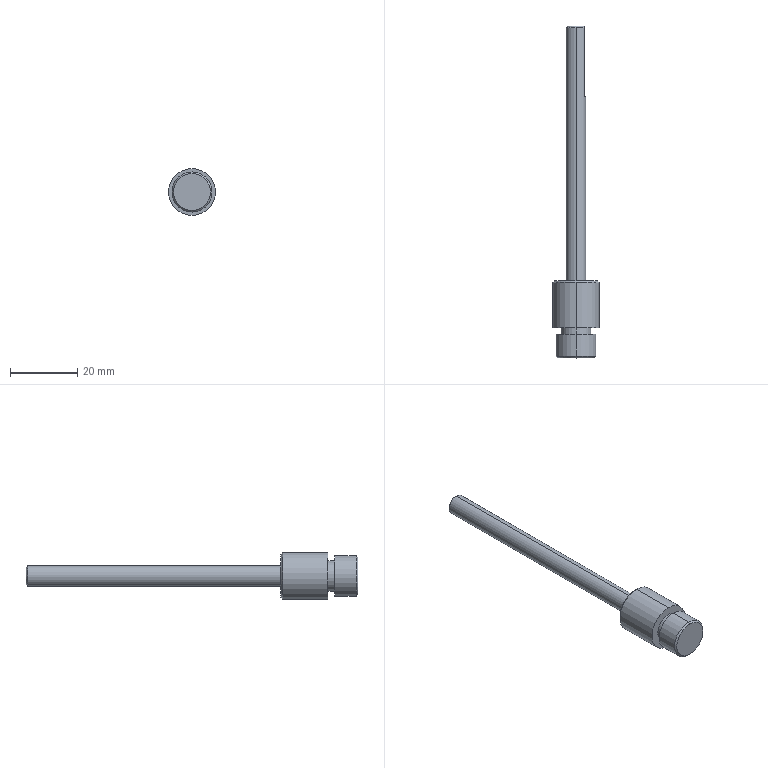Part | STEP file | 1 solid | 22 faces | box 14 x 99 x 14 mm | volume 5187 mm3 | cylinder 8 | cone 7 | plane 7 | commonest cylinder face diameters 6 x2 9 x2 12 x2 14 x2
STEP:
#1=CARTESIAN_POINT('',(0.,0.,0.));
#2=DIRECTION('',(0.,0.,1.));
#3=DIRECTION('',(1.,0.,0.));
#4=AXIS2_PLACEMENT_3D('',#1,#2,#3);
#5=CARTESIAN_POINT('',(0.,-9.,-5.5));
#6=VERTEX_POINT('',#5);
#7=CARTESIAN_POINT('',(0.,-9.,5.5));
#8=VERTEX_POINT('',#7);
#9=CARTESIAN_POINT('',(0.,-9.,0.));
#10=DIRECTION('',(0.,-1.,0.));
#11=DIRECTION('',(0.,0.,-1.));
#12=AXIS2_PLACEMENT_3D('',#9,#10,#11);
#13=CIRCLE('',#12,5.5);
#14=CARTESIAN_POINT('',(0.,-9.,0.));
#15=DIRECTION('',(0.,1.,0.));
#16=DIRECTION('',(0.,0.,1.));
#17=AXIS2_PLACEMENT_3D('',#14,#15,#16);
#18=CONICAL_SURFACE('',#17,5.5,0.7854);
#19=CARTESIAN_POINT('',(3.142,0.));
#20=DIRECTION('',(-1.,0.));
#21=VECTOR('',#20,1.);
#22=LINE('',#19,#21);
#23=(GEOMETRIC_REPRESENTATION_CONTEXT(2)PARAMETRIC_REPRESENTATION_CONTEXT()REPRESENTATION_CONTEXT('',''));
#24=DEFINITIONAL_REPRESENTATION('',(#22),#23);
#25=PCURVE('',#18,#24);
#26=CARTESIAN_POINT('',(0.,-9.,0.));
#27=DIRECTION('',(0.,-1.,0.));
#28=DIRECTION('',(0.,0.,-1.));
#29=AXIS2_PLACEMENT_3D('',#26,#27,#28);
#30=PLANE('',#29);
#31=CARTESIAN_POINT('',(0.,0.));
#32=DIRECTION('',(1.,0.));
#33=AXIS2_PLACEMENT_2D('',#31,#32);
#34=CIRCLE('',#33,5.5);
#35=(GEOMETRIC_REPRESENTATION_CONTEXT(2)PARAMETRIC_REPRESENTATION_CONTEXT()REPRESENTATION_CONTEXT('',''));
#36=DEFINITIONAL_REPRESENTATION('',(#34),#35);
#37=PCURVE('',#30,#36);
#38=SURFACE_CURVE('',#13,(#25,#37),.PCURVE_S1.);
#39=EDGE_CURVE('',#6,#8,#38,.T.);
#40=ORIENTED_EDGE('',*,*,#39,.F.);
#41=CARTESIAN_POINT('',(0.,-8.5,-6.));
#42=VERTEX_POINT('',#41);
#43=CARTESIAN_POINT('',(0.,-9.,-5.5));
#44=DIRECTION('',(0.,0.7071,-0.7071));
#45=VECTOR('',#44,1.);
#46=LINE('',#43,#45);
#47=CARTESIAN_POINT('',(3.142,0.));
#48=DIRECTION('',(0.,1.));
#49=VECTOR('',#48,1.);
#50=LINE('',#47,#49);
#51=(GEOMETRIC_REPRESENTATION_CONTEXT(2)PARAMETRIC_REPRESENTATION_CONTEXT()REPRESENTATION_CONTEXT('',''));
#52=DEFINITIONAL_REPRESENTATION('',(#50),#51);
#53=PCURVE('',#18,#52);
#54=CARTESIAN_POINT('',(0.,-9.,0.));
#55=DIRECTION('',(0.,1.,0.));
#56=DIRECTION('',(0.,0.,1.));
#57=AXIS2_PLACEMENT_3D('',#54,#55,#56);
#58=CONICAL_SURFACE('',#57,5.5,0.7854);
#59=CARTESIAN_POINT('',(3.142,0.));
#60=DIRECTION('',(0.,1.));
#61=VECTOR('',#60,1.);
#62=LINE('',#59,#61);
#63=(GEOMETRIC_REPRESENTATION_CONTEXT(2)PARAMETRIC_REPRESENTATION_CONTEXT()REPRESENTATION_CONTEXT('',''));
#64=DEFINITIONAL_REPRESENTATION('',(#62),#63);
#65=PCURVE('',#58,#64);
#66=SURFACE_CURVE('',#46,(#53,#65),.PCURVE_S1.);
#67=EDGE_CURVE('',#6,#42,#66,.T.);
#68=ORIENTED_EDGE('',*,*,#67,.T.);
#69=CARTESIAN_POINT('',(0.,-8.5,6.));
#70=VERTEX_POINT('',#69);
#71=CARTESIAN_POINT('',(0.,-8.5,0.));
#72=DIRECTION('',(0.,1.,0.));
#73=DIRECTION('',(0.,0.,-1.));
#74=AXIS2_PLACEMENT_3D('',#71,#72,#73);
#75=CIRCLE('',#74,6.);
#76=CARTESIAN_POINT('',(-3.142,0.5));
#77=DIRECTION('',(1.,0.));
#78=VECTOR('',#77,1.);
#79=LINE('',#76,#78);
#80=(GEOMETRIC_REPRESENTATION_CONTEXT(2)PARAMETRIC_REPRESENTATION_CONTEXT()REPRESENTATION_CONTEXT('',''));
#81=DEFINITIONAL_REPRESENTATION('',(#79),#80);
#82=PCURVE('',#18,#81);
#83=CARTESIAN_POINT('',(0.,-9.,0.));
#84=DIRECTION('',(0.,1.,0.));
#85=DIRECTION('',(0.,0.,1.));
#86=AXIS2_PLACEMENT_3D('',#83,#84,#85);
#87=CYLINDRICAL_SURFACE('',#86,6.);
#88=CARTESIAN_POINT('',(-3.142,0.5));
#89=DIRECTION('',(1.,0.));
#90=VECTOR('',#89,1.);
#91=LINE('',#88,#90);
#92=(GEOMETRIC_REPRESENTATION_CONTEXT(2)PARAMETRIC_REPRESENTATION_CONTEXT()REPRESENTATION_CONTEXT('',''));
#93=DEFINITIONAL_REPRESENTATION('',(#91),#92);
#94=PCURVE('',#87,#93);
#95=SURFACE_CURVE('',#75,(#82,#94),.PCURVE_S1.);
#96=EDGE_CURVE('',#70,#42,#95,.T.);
#97=ORIENTED_EDGE('',*,*,#96,.F.);
#98=CARTESIAN_POINT('',(0.,-9.,5.5));
#99=DIRECTION('',(0.,0.7071,0.7071));
#100=VECTOR('',#99,1.);
#101=LINE('',#98,#100);
#102=CARTESIAN_POINT('',(0.,0.));
#103=DIRECTION('',(0.,1.));
#104=VECTOR('',#103,1.);
#105=LINE('',#102,#104);
#106=(GEOMETRIC_REPRESENTATION_CONTEXT(2)PARAMETRIC_REPRESENTATION_CONTEXT()REPRESENTATION_CONTEXT('',''));
#107=DEFINITIONAL_REPRESENTATION('',(#105),#106);
#108=PCURVE('',#18,#107);
#109=CARTESIAN_POINT('',(6.283,0.));
#110=DIRECTION('',(0.,1.));
#111=VECTOR('',#110,1.);
#112=LINE('',#109,#111);
#113=(GEOMETRIC_REPRESENTATION_CONTEXT(2)PARAMETRIC_REPRESENTATION_CONTEXT()REPRESENTATION_CONTEXT('',''));
#114=DEFINITIONAL_REPRESENTATION('',(#112),#113);
#115=PCURVE('',#58,#114);
#116=SURFACE_CURVE('',#101,(#108,#115),.PCURVE_S1.);
#117=EDGE_CURVE('',#8,#70,#116,.T.);
#118=ORIENTED_EDGE('',*,*,#117,.F.);
#119=EDGE_LOOP('',(#40,#68,#97,#118));
#120=FACE_BOUND('',#119,.T.);
#121=ADVANCED_FACE('',(#120),#18,.T.);
#122=CARTESIAN_POINT('',(0.,14.,6.5));
#123=VERTEX_POINT('',#122);
#124=CARTESIAN_POINT('',(0.,14.,-6.5));
#125=VERTEX_POINT('',#124);
#126=CARTESIAN_POINT('',(0.,14.,0.));
#127=DIRECTION('',(0.,1.,0.));
#128=DIRECTION('',(0.,0.,1.));
#129=AXIS2_PLACEMENT_3D('',#126,#127,#128);
#130=CIRCLE('',#129,6.5);
#131=CARTESIAN_POINT('',(0.,14.,0.));
#132=DIRECTION('',(0.,-1.,0.));
#133=DIRECTION('',(0.,0.,-1.));
#134=AXIS2_PLACEMENT_3D('',#131,#132,#133);
#135=CONICAL_SURFACE('',#134,6.5,0.7854);
#136=CARTESIAN_POINT('',(3.142,0.));
#137=DIRECTION('',(-1.,0.));
#138=VECTOR('',#137,1.);
#139=LINE('',#136,#138);
#140=(GEOMETRIC_REPRESENTATION_CONTEXT(2)PARAMETRIC_REPRESENTATION_CONTEXT()REPRESENTATION_CONTEXT('',''));
#141=DEFINITIONAL_REPRESENTATION('',(#139),#140);
#142=PCURVE('',#135,#141);
#143=CARTESIAN_POINT('',(0.,14.,0.));
#144=DIRECTION('',(0.,1.,0.));
#145=DIRECTION('',(0.,0.,1.));
#146=AXIS2_PLACEMENT_3D('',#143,#144,#145);
#147=PLANE('',#146);
#148=CARTESIAN_POINT('',(0.,0.));
#149=DIRECTION('',(1.,0.));
#150=AXIS2_PLACEMENT_2D('',#148,#149);
#151=CIRCLE('',#150,6.5);
#152=(GEOMETRIC_REPRESENTATION_CONTEXT(2)PARAMETRIC_REPRESENTATION_CONTEXT()REPRESENTATION_CONTEXT('',''));
#153=DEFINITIONAL_REPRESENTATION('',(#151),#152);
#154=PCURVE('',#147,#153);
#155=SURFACE_CURVE('',#130,(#142,#154),.PCURVE_S1.);
#156=EDGE_CURVE('',#123,#125,#155,.T.);
#157=ORIENTED_EDGE('',*,*,#156,.F.);
#158=CARTESIAN_POINT('',(0.,13.5,7.));
#159=VERTEX_POINT('',#158);
#160=CARTESIAN_POINT('',(0.,14.,6.5));
#161=DIRECTION('',(0.,-0.7071,0.7071));
#162=VECTOR('',#161,1.);
#163=LINE('',#160,#162);
#164=CARTESIAN_POINT('',(3.142,0.));
#165=DIRECTION('',(0.,1.));
#166=VECTOR('',#165,1.);
#167=LINE('',#164,#166);
#168=(GEOMETRIC_REPRESENTATION_CONTEXT(2)PARAMETRIC_REPRESENTATION_CONTEXT()REPRESENTATION_CONTEXT('',''));
#169=DEFINITIONAL_REPRESENTATION('',(#167),#168);
#170=PCURVE('',#135,#169);
#171=CARTESIAN_POINT('',(0.,14.,0.));
#172=DIRECTION('',(0.,-1.,0.));
#173=DIRECTION('',(0.,0.,-1.));
#174=AXIS2_PLACEMENT_3D('',#171,#172,#173);
#175=CONICAL_SURFACE('',#174,6.5,0.7854);
#176=CARTESIAN_POINT('',(3.142,0.));
#177=DIRECTION('',(0.,1.));
#178=VECTOR('',#177,1.);
#179=LINE('',#176,#178);
#180=(GEOMETRIC_REPRESENTATION_CONTEXT(2)PARAMETRIC_REPRESENTATION_CONTEXT()REPRESENTATION_CONTEXT('',''));
#181=DEFINITIONAL_REPRESENTATION('',(#179),#180);
#182=PCURVE('',#175,#181);
#183=SURFACE_CURVE('',#163,(#170,#182),.PCURVE_S1.);
#184=EDGE_CURVE('',#123,#159,#183,.T.);
#185=ORIENTED_EDGE('',*,*,#184,.T.);
#186=CARTESIAN_POINT('',(0.,13.5,-7.));
#187=VERTEX_POINT('',#186);
#188=CARTESIAN_POINT('',(0.,13.5,0.));
#189=DIRECTION('',(0.,-1.,0.));
#190=DIRECTION('',(0.,0.,1.));
#191=AXIS2_PLACEMENT_3D('',#188,#189,#190);
#192=CIRCLE('',#191,7.);
#193=CARTESIAN_POINT('',(-3.142,0.5));
#194=DIRECTION('',(1.,0.));
#195=VECTOR('',#194,1.);
#196=LINE('',#193,#195);
#197=(GEOMETRIC_REPRESENTATION_CONTEXT(2)PARAMETRIC_REPRESENTATION_CONTEXT()REPRESENTATION_CONTEXT('',''));
#198=DEFINITIONAL_REPRESENTATION('',(#196),#197);
#199=PCURVE('',#135,#198);
#200=CARTESIAN_POINT('',(0.,14.,0.));
#201=DIRECTION('',(0.,-1.,0.));
#202=DIRECTION('',(0.,0.,-1.));
#203=AXIS2_PLACEMENT_3D('',#200,#201,#202);
#204=CYLINDRICAL_SURFACE('',#203,7.);
#205=CARTESIAN_POINT('',(-3.142,0.5));
#206=DIRECTION('',(1.,0.));
#207=VECTOR('',#206,1.);
#208=LINE('',#205,#207);
#209=(GEOMETRIC_REPRESENTATION_CONTEXT(2)PARAMETRIC_REPRESENTATION_CONTEXT()REPRESENTATION_CONTEXT('',''));
#210=DEFINITIONAL_REPRESENTATION('',(#208),#209);
#211=PCURVE('',#204,#210);
#212=SURFACE_CURVE('',#192,(#199,#211),.PCURVE_S1.);
#213=EDGE_CURVE('',#187,#159,#212,.T.);
#214=ORIENTED_EDGE('',*,*,#213,.F.);
#215=CARTESIAN_POINT('',(0.,14.,-6.5));
#216=DIRECTION('',(0.,-0.7071,-0.7071));
#217=VECTOR('',#216,1.);
#218=LINE('',#215,#217);
#219=CARTESIAN_POINT('',(0.,0.));
#220=DIRECTION('',(0.,1.));
#221=VECTOR('',#220,1.);
#222=LINE('',#219,#221);
#223=(GEOMETRIC_REPRESENTATION_CONTEXT(2)PARAMETRIC_REPRESENTATION_CONTEXT()REPRESENTATION_CONTEXT('',''));
#224=DEFINITIONAL_REPRESENTATION('',(#222),#223);
#225=PCURVE('',#135,#224);
#226=CARTESIAN_POINT('',(6.283,0.));
#227=DIRECTION('',(0.,1.));
#228=VECTOR('',#227,1.);
#229=LINE('',#226,#228);
#230=(GEOMETRIC_REPRESENTATION_CONTEXT(2)PARAMETRIC_REPRESENTATION_CONTEXT()REPRESENTATION_CONTEXT('',''));
#231=DEFINITIONAL_REPRESENTATION('',(#229),#230);
#232=PCURVE('',#175,#231);
#233=SURFACE_CURVE('',#218,(#225,#232),.PCURVE_S1.);
#234=EDGE_CURVE('',#125,#187,#233,.T.);
#235=ORIENTED_EDGE('',*,*,#234,.F.);
#236=EDGE_LOOP('',(#157,#185,#214,#235));
#237=FACE_BOUND('',#236,.T.);
#238=ADVANCED_FACE('',(#237),#135,.T.);
#239=CARTESIAN_POINT('',(0.,90.,2.5));
#240=VERTEX_POINT('',#239);
#241=CARTESIAN_POINT('',(2.5,90.,0.));
#242=VERTEX_POINT('',#241);
#243=CARTESIAN_POINT('',(0.,90.,0.));
#244=DIRECTION('',(0.,1.,0.));
#245=DIRECTION('',(0.,0.,1.));
#246=AXIS2_PLACEMENT_3D('',#243,#244,#245);
#247=CIRCLE('',#246,2.5);
#248=CARTESIAN_POINT('',(0.,90.,0.));
#249=DIRECTION('',(0.,-1.,0.));
#250=DIRECTION('',(0.,0.,-1.));
#251=AXIS2_PLACEMENT_3D('',#248,#249,#250);
#252=CONICAL_SURFACE('',#251,2.5,0.7854);
#253=CARTESIAN_POINT('',(3.142,0.));
#254=DIRECTION('',(-1.,0.));
#255=VECTOR('',#254,1.);
#256=LINE('',#253,#255);
#257=(GEOMETRIC_REPRESENTATION_CONTEXT(2)PARAMETRIC_REPRESENTATION_CONTEXT()REPRESENTATION_CONTEXT('',''));
#258=DEFINITIONAL_REPRESENTATION('',(#256),#257);
#259=PCURVE('',#252,#258);
#260=CARTESIAN_POINT('',(0.,90.,0.));
#261=DIRECTION('',(0.,1.,0.));
#262=DIRECTION('',(0.,0.,1.));
#263=AXIS2_PLACEMENT_3D('',#260,#261,#262);
#264=PLANE('',#263);
#265=CARTESIAN_POINT('',(0.,0.));
#266=DIRECTION('',(1.,0.));
#267=AXIS2_PLACEMENT_2D('',#265,#266);
#268=CIRCLE('',#267,2.5);
#269=(GEOMETRIC_REPRESENTATION_CONTEXT(2)PARAMETRIC_REPRESENTATION_CONTEXT()REPRESENTATION_CONTEXT('',''));
#270=DEFINITIONAL_REPRESENTATION('',(#268),#269);
#271=PCURVE('',#264,#270);
#272=SURFACE_CURVE('',#247,(#259,#271),.PCURVE_S1.);
#273=EDGE_CURVE('',#240,#242,#272,.T.);
#274=ORIENTED_EDGE('',*,*,#273,.F.);
#275=CARTESIAN_POINT('',(0.,89.5,3.));
#276=VERTEX_POINT('',#275);
#277=CARTESIAN_POINT('',(0.,90.,2.5));
#278=DIRECTION('',(0.,-0.7071,0.7071));
#279=VECTOR('',#278,1.);
#280=LINE('',#277,#279);
#281=CARTESIAN_POINT('',(3.142,0.));
#282=DIRECTION('',(0.,1.));
#283=VECTOR('',#282,1.);
#284=LINE('',#281,#283);
#285=(GEOMETRIC_REPRESENTATION_CONTEXT(2)PARAMETRIC_REPRESENTATION_CONTEXT()REPRESENTATION_CONTEXT('',''));
#286=DEFINITIONAL_REPRESENTATION('',(#284),#285);
#287=PCURVE('',#252,#286);
#288=CARTESIAN_POINT('',(0.,90.,0.));
#289=DIRECTION('',(0.,-1.,0.));
#290=DIRECTION('',(0.,0.,-1.));
#291=AXIS2_PLACEMENT_3D('',#288,#289,#290);
#292=CONICAL_SURFACE('',#291,2.5,0.7854);
#293=CARTESIAN_POINT('',(3.142,0.));
#294=DIRECTION('',(0.,1.));
#295=VECTOR('',#294,1.);
#296=LINE('',#293,#295);
#297=(GEOMETRIC_REPRESENTATION_CONTEXT(2)PARAMETRIC_REPRESENTATION_CONTEXT()REPRESENTATION_CONTEXT('',''));
#298=DEFINITIONAL_REPRESENTATION('',(#296),#297);
#299=PCURVE('',#292,#298);
#300=SURFACE_CURVE('',#280,(#287,#299),.PCURVE_S1.);
#301=EDGE_CURVE('',#240,#276,#300,.T.);
#302=ORIENTED_EDGE('',*,*,#301,.T.);
#303=CARTESIAN_POINT('',(2.5,89.5,1.658));
#304=VERTEX_POINT('',#303);
#305=CARTESIAN_POINT('',(0.,89.5,0.));
#306=DIRECTION('',(0.,-1.,0.));
#307=DIRECTION('',(0.,0.,1.));
#308=AXIS2_PLACEMENT_3D('',#305,#306,#307);
#309=CIRCLE('',#308,3.);
#310=CARTESIAN_POINT('',(-3.142,0.5));
#311=DIRECTION('',(1.,0.));
#312=VECTOR('',#311,1.);
#313=LINE('',#310,#312);
#314=(GEOMETRIC_REPRESENTATION_CONTEXT(2)PARAMETRIC_REPRESENTATION_CONTEXT()REPRESENTATION_CONTEXT('',''));
#315=DEFINITIONAL_REPRESENTATION('',(#313),#314);
#316=PCURVE('',#252,#315);
#317=CARTESIAN_POINT('',(0.,90.,0.));
#318=DIRECTION('',(0.,-1.,0.));
#319=DIRECTION('',(0.,0.,-1.));
#320=AXIS2_PLACEMENT_3D('',#317,#318,#319);
#321=CYLINDRICAL_SURFACE('',#320,3.);
#322=CARTESIAN_POINT('',(-3.142,0.5));
#323=DIRECTION('',(1.,0.));
#324=VECTOR('',#323,1.);
#325=LINE('',#322,#324);
#326=(GEOMETRIC_REPRESENTATION_CONTEXT(2)PARAMETRIC_REPRESENTATION_CONTEXT()REPRESENTATION_CONTEXT('',''));
#327=DEFINITIONAL_REPRESENTATION('',(#325),#326);
#328=PCURVE('',#321,#327);
#329=SURFACE_CURVE('',#309,(#316,#328),.PCURVE_S1.);
#330=EDGE_CURVE('',#304,#276,#329,.T.);
#331=ORIENTED_EDGE('',*,*,#330,.F.);
#332=CARTESIAN_POINT('',(2.5,90.,0.));
#333=CARTESIAN_POINT('',(2.5,90.,0.2944));
#334=CARTESIAN_POINT('',(2.5,89.947,0.5796));
#335=CARTESIAN_POINT('',(2.5,89.766,1.137));
#336=CARTESIAN_POINT('',(2.5,89.642,1.402));
#337=CARTESIAN_POINT('',(2.5,89.5,1.658));
#338=B_SPLINE_CURVE_WITH_KNOTS('',3,(#332,#333,#334,#335,#336,#337),.UNSPECIFIED.,.F.,.F.,(4,2,4),(0.,0.0008701,0.00174),.UNSPECIFIED.);
#339=CARTESIAN_POINT('',(1.571,0.));
#340=CARTESIAN_POINT('',(1.582,-0.000000235));
#341=CARTESIAN_POINT('',(1.603,0.0008657));
#342=CARTESIAN_POINT('',(1.635,0.004703));
#343=CARTESIAN_POINT('',(1.666,0.01102));
#344=CARTESIAN_POINT('',(1.697,0.01975));
#345=CARTESIAN_POINT('',(1.728,0.03084));
#346=CARTESIAN_POINT('',(1.758,0.04421));
#347=CARTESIAN_POINT('',(1.788,0.0598));
#348=CARTESIAN_POINT('',(1.817,0.07753));
#349=CARTESIAN_POINT('',(1.846,0.09734));
#350=CARTESIAN_POINT('',(1.874,0.1191));
#351=CARTESIAN_POINT('',(1.902,0.1429));
#352=CARTESIAN_POINT('',(1.928,0.1685));
#353=CARTESIAN_POINT('',(1.954,0.1956));
#354=CARTESIAN_POINT('',(1.98,0.2243));
#355=CARTESIAN_POINT('',(2.004,0.2545));
#356=CARTESIAN_POINT('',(2.028,0.286));
#357=CARTESIAN_POINT('',(2.051,0.3188));
#358=CARTESIAN_POINT('',(2.074,0.3529));
#359=CARTESIAN_POINT('',(2.095,0.3881));
#360=CARTESIAN_POINT('',(2.116,0.4244));
#361=CARTESIAN_POINT('',(2.137,0.4616));
#362=CARTESIAN_POINT('',(2.15,0.4871));
#363=CARTESIAN_POINT('',(2.156,0.5));
#364=B_SPLINE_CURVE_WITH_KNOTS('',3,(#339,#340,#341,#342,#343,#344,#345,#346,#347,#348,#349,#350,#351,#352,#353,#354,#355,#356,#357,#358,#359,#360,#361,#362,#363),.UNSPECIFIED.,.F.,.F.,(4,1,1,1,1,1,1,1,1,1,1,1,1,1,1,1,1,1,1,1,1,1,4),(0.,0.0000791,0.0001582,0.0002373,0.0003164,0.0003955,0.0004746,0.0005537,0.0006328,0.0007119,0.000791,0.0008701,0.0009492,0.001028,0.001107,0.001186,0.001266,0.001345,0.001424,0.001503,0.001582,0.001661,0.00174),.QUASI_UNIFORM_KNOTS.);
#365=(GEOMETRIC_REPRESENTATION_CONTEXT(2)PARAMETRIC_REPRESENTATION_CONTEXT()REPRESENTATION_CONTEXT('',''));
#366=DEFINITIONAL_REPRESENTATION('',(#364),#365);
#367=PCURVE('',#252,#366);
#368=CARTESIAN_POINT('',(2.5,90.,-3.));
#369=DIRECTION('',(-1.,0.,0.));
#370=DIRECTION('',(0.,-1.,0.));
#371=AXIS2_PLACEMENT_3D('',#368,#369,#370);
#372=PLANE('',#371);
#373=CARTESIAN_POINT('',(0.,3.));
#374=CARTESIAN_POINT('',(0.,3.294));
#375=CARTESIAN_POINT('',(0.05273,3.58));
#376=CARTESIAN_POINT('',(0.2337,4.137));
#377=CARTESIAN_POINT('',(0.3583,4.402));
#378=CARTESIAN_POINT('',(0.5,4.658));
#379=B_SPLINE_CURVE_WITH_KNOTS('',3,(#373,#374,#375,#376,#377,#378),.UNSPECIFIED.,.F.,.F.,(4,2,4),(0.,0.0008701,0.00174),.UNSPECIFIED.);
#380=(GEOMETRIC_REPRESENTATION_CONTEXT(2)PARAMETRIC_REPRESENTATION_CONTEXT()REPRESENTATION_CONTEXT('',''));
#381=DEFINITIONAL_REPRESENTATION('',(#379),#380);
#382=PCURVE('',#372,#381);
#383=SURFACE_CURVE('',#338,(#367,#382),.PCURVE_S1.);
#384=EDGE_CURVE('',#242,#304,#383,.T.);
#385=ORIENTED_EDGE('',*,*,#384,.F.);
#386=EDGE_LOOP('',(#274,#302,#331,#385));
#387=FACE_BOUND('',#386,.T.);
#388=ADVANCED_FACE('',(#387),#252,.T.);
#389=ORIENTED_EDGE('',*,*,#301,.F.);
#390=CARTESIAN_POINT('',(0.,90.,-2.5));
#391=VERTEX_POINT('',#390);
#392=CARTESIAN_POINT('',(0.,90.,0.));
#393=DIRECTION('',(0.,1.,0.));
#394=DIRECTION('',(0.,0.,1.));
#395=AXIS2_PLACEMENT_3D('',#392,#393,#394);
#396=CIRCLE('',#395,2.5);
#397=CARTESIAN_POINT('',(9.425,0.));
#398=DIRECTION('',(-1.,0.));
#399=VECTOR('',#398,1.);
#400=LINE('',#397,#399);
#401=(GEOMETRIC_REPRESENTATION_CONTEXT(2)PARAMETRIC_REPRESENTATION_CONTEXT()REPRESENTATION_CONTEXT('',''));
#402=DEFINITIONAL_REPRESENTATION('',(#400),#401);
#403=PCURVE('',#292,#402);
#404=CARTESIAN_POINT('',(0.,0.));
#405=DIRECTION('',(1.,0.));
#406=AXIS2_PLACEMENT_2D('',#404,#405);
#407=CIRCLE('',#406,2.5);
#408=(GEOMETRIC_REPRESENTATION_CONTEXT(2)PARAMETRIC_REPRESENTATION_CONTEXT()REPRESENTATION_CONTEXT('',''));
#409=DEFINITIONAL_REPRESENTATION('',(#407),#408);
#410=PCURVE('',#264,#409);
#411=SURFACE_CURVE('',#396,(#403,#410),.PCURVE_S1.);
#412=EDGE_CURVE('',#391,#240,#411,.T.);
#413=ORIENTED_EDGE('',*,*,#412,.F.);
#414=CARTESIAN_POINT('',(0.,89.5,-3.));
#415=VERTEX_POINT('',#414);
#416=CARTESIAN_POINT('',(0.,90.,-2.5));
#417=DIRECTION('',(0.,-0.7071,-0.7071));
#418=VECTOR('',#417,1.);
#419=LINE('',#416,#418);
#420=CARTESIAN_POINT('',(6.283,0.));
#421=DIRECTION('',(0.,1.));
#422=VECTOR('',#421,1.);
#423=LINE('',#420,#422);
#424=(GEOMETRIC_REPRESENTATION_CONTEXT(2)PARAMETRIC_REPRESENTATION_CONTEXT()REPRESENTATION_CONTEXT('',''));
#425=DEFINITIONAL_REPRESENTATION('',(#423),#424);
#426=PCURVE('',#292,#425);
#427=CARTESIAN_POINT('',(0.,90.,0.));
#428=DIRECTION('',(0.,-1.,0.));
#429=DIRECTION('',(0.,0.,-1.));
#430=AXIS2_PLACEMENT_3D('',#427,#428,#429);
#431=CONICAL_SURFACE('',#430,2.5,0.7854);
#432=CARTESIAN_POINT('',(0.,0.));
#433=DIRECTION('',(0.,1.));
#434=VECTOR('',#433,1.);
#435=LINE('',#432,#434);
#436=(GEOMETRIC_REPRESENTATION_CONTEXT(2)PARAMETRIC_REPRESENTATION_CONTEXT()REPRESENTATION_CONTEXT('',''));
#437=DEFINITIONAL_REPRESENTATION('',(#435),#436);
#438=PCURVE('',#431,#437);
#439=SURFACE_CURVE('',#419,(#426,#438),.PCURVE_S1.);
#440=EDGE_CURVE('',#391,#415,#439,.T.);
#441=ORIENTED_EDGE('',*,*,#440,.T.);
#442=CARTESIAN_POINT('',(0.,89.5,0.));
#443=DIRECTION('',(0.,-1.,0.));
#444=DIRECTION('',(0.,0.,1.));
#445=AXIS2_PLACEMENT_3D('',#442,#443,#444);
#446=CIRCLE('',#445,3.);
#447=CARTESIAN_POINT('',(3.142,0.5));
#448=DIRECTION('',(1.,0.));
#449=VECTOR('',#448,1.);
#450=LINE('',#447,#449);
#451=(GEOMETRIC_REPRESENTATION_CONTEXT(2)PARAMETRIC_REPRESENTATION_CONTEXT()REPRESENTATION_CONTEXT('',''));
#452=DEFINITIONAL_REPRESENTATION('',(#450),#451);
#453=PCURVE('',#292,#452);
#454=CARTESIAN_POINT('',(0.,90.,0.));
#455=DIRECTION('',(0.,-1.,0.));
#456=DIRECTION('',(0.,0.,-1.));
#457=AXIS2_PLACEMENT_3D('',#454,#455,#456);
#458=CYLINDRICAL_SURFACE('',#457,3.);
#459=CARTESIAN_POINT('',(3.142,0.5));
#460=DIRECTION('',(1.,0.));
#461=VECTOR('',#460,1.);
#462=LINE('',#459,#461);
#463=(GEOMETRIC_REPRESENTATION_CONTEXT(2)PARAMETRIC_REPRESENTATION_CONTEXT()REPRESENTATION_CONTEXT('',''));
#464=DEFINITIONAL_REPRESENTATION('',(#462),#463);
#465=PCURVE('',#458,#464);
#466=SURFACE_CURVE('',#446,(#453,#465),.PCURVE_S1.);
#467=EDGE_CURVE('',#276,#415,#466,.T.);
#468=ORIENTED_EDGE('',*,*,#467,.F.);
#469=EDGE_LOOP('',(#389,#413,#441,#468));
#470=FACE_BOUND('',#469,.T.);
#471=ADVANCED_FACE('',(#470),#292,.T.);
#472=ORIENTED_EDGE('',*,*,#96,.T.);
#473=CARTESIAN_POINT('',(0.,-2.,-6.));
#474=VERTEX_POINT('',#473);
#475=CARTESIAN_POINT('',(0.,-9.,-6.));
#476=DIRECTION('',(0.,1.,0.));
#477=VECTOR('',#476,1.);
#478=LINE('',#475,#477);
#479=CARTESIAN_POINT('',(3.142,0.));
#480=DIRECTION('',(0.,1.));
#481=VECTOR('',#480,1.);
#482=LINE('',#479,#481);
#483=(GEOMETRIC_REPRESENTATION_CONTEXT(2)PARAMETRIC_REPRESENTATION_CONTEXT()REPRESENTATION_CONTEXT('',''));
#484=DEFINITIONAL_REPRESENTATION('',(#482),#483);
#485=PCURVE('',#87,#484);
#486=CARTESIAN_POINT('',(0.,-9.,0.));
#487=DIRECTION('',(0.,1.,0.));
#488=DIRECTION('',(0.,0.,1.));
#489=AXIS2_PLACEMENT_3D('',#486,#487,#488);
#490=CYLINDRICAL_SURFACE('',#489,6.);
#491=CARTESIAN_POINT('',(3.142,0.));
#492=DIRECTION('',(0.,1.));
#493=VECTOR('',#492,1.);
#494=LINE('',#491,#493);
#495=(GEOMETRIC_REPRESENTATION_CONTEXT(2)PARAMETRIC_REPRESENTATION_CONTEXT()REPRESENTATION_CONTEXT('',''));
#496=DEFINITIONAL_REPRESENTATION('',(#494),#495);
#497=PCURVE('',#490,#496);
#498=SURFACE_CURVE('',#478,(#485,#497),.PCURVE_S1.);
#499=EDGE_CURVE('',#42,#474,#498,.T.);
#500=ORIENTED_EDGE('',*,*,#499,.T.);
#501=CARTESIAN_POINT('',(0.,-2.,6.));
#502=VERTEX_POINT('',#501);
#503=CARTESIAN_POINT('',(0.,-2.,0.));
#504=DIRECTION('',(0.,-1.,0.));
#505=DIRECTION('',(0.,0.,-1.));
#506=AXIS2_PLACEMENT_3D('',#503,#504,#505);
#507=CIRCLE('',#506,6.);
#508=CARTESIAN_POINT('',(3.142,7.));
#509=DIRECTION('',(-1.,0.));
#510=VECTOR('',#509,1.);
#511=LINE('',#508,#510);
#512=(GEOMETRIC_REPRESENTATION_CONTEXT(2)PARAMETRIC_REPRESENTATION_CONTEXT()REPRESENTATION_CONTEXT('',''));
#513=DEFINITIONAL_REPRESENTATION('',(#511),#512);
#514=PCURVE('',#87,#513);
#515=CARTESIAN_POINT('',(0.,-2.,0.));
#516=DIRECTION('',(0.,-1.,0.));
#517=DIRECTION('',(0.,0.,-1.));
#518=AXIS2_PLACEMENT_3D('',#515,#516,#517);
#519=PLANE('',#518);
#520=CARTESIAN_POINT('',(0.,0.));
#521=DIRECTION('',(1.,0.));
#522=AXIS2_PLACEMENT_2D('',#520,#521);
#523=CIRCLE('',#522,6.);
#524=(GEOMETRIC_REPRESENTATION_CONTEXT(2)PARAMETRIC_REPRESENTATION_CONTEXT()REPRESENTATION_CONTEXT('',''));
#525=DEFINITIONAL_REPRESENTATION('',(#523),#524);
#526=PCURVE('',#519,#525);
#527=SURFACE_CURVE('',#507,(#514,#526),.PCURVE_S1.);
#528=EDGE_CURVE('',#474,#502,#527,.T.);
#529=ORIENTED_EDGE('',*,*,#528,.T.);
#530=CARTESIAN_POINT('',(0.,-9.,6.));
#531=DIRECTION('',(0.,1.,0.));
#532=VECTOR('',#531,1.);
#533=LINE('',#530,#532);
#534=CARTESIAN_POINT('',(0.,0.));
#535=DIRECTION('',(0.,1.));
#536=VECTOR('',#535,1.);
#537=LINE('',#534,#536);
#538=(GEOMETRIC_REPRESENTATION_CONTEXT(2)PARAMETRIC_REPRESENTATION_CONTEXT()REPRESENTATION_CONTEXT('',''));
#539=DEFINITIONAL_REPRESENTATION('',(#537),#538);
#540=PCURVE('',#87,#539);
#541=CARTESIAN_POINT('',(6.283,0.));
#542=DIRECTION('',(0.,1.));
#543=VECTOR('',#542,1.);
#544=LINE('',#541,#543);
#545=(GEOMETRIC_REPRESENTATION_CONTEXT(2)PARAMETRIC_REPRESENTATION_CONTEXT()REPRESENTATION_CONTEXT('',''));
#546=DEFINITIONAL_REPRESENTATION('',(#544),#545);
#547=PCURVE('',#490,#546);
#548=SURFACE_CURVE('',#533,(#540,#547),.PCURVE_S1.);
#549=EDGE_CURVE('',#70,#502,#548,.T.);
#550=ORIENTED_EDGE('',*,*,#549,.F.);
#551=EDGE_LOOP('',(#472,#500,#529,#550));
#552=FACE_BOUND('',#551,.T.);
#553=ADVANCED_FACE('',(#552),#87,.T.);
#554=CARTESIAN_POINT('',(0.,-2.,-4.5));
#555=VERTEX_POINT('',#554);
#556=CARTESIAN_POINT('',(0.,-2.,4.5));
#557=VERTEX_POINT('',#556);
#558=CARTESIAN_POINT('',(0.,-2.,0.));
#559=DIRECTION('',(0.,-1.,0.));
#560=DIRECTION('',(0.,0.,-1.));
#561=AXIS2_PLACEMENT_3D('',#558,#559,#560);
#562=CIRCLE('',#561,4.5);
#563=CARTESIAN_POINT('',(0.,-2.,0.));
#564=DIRECTION('',(0.,1.,0.));
#565=DIRECTION('',(0.,0.,1.));
#566=AXIS2_PLACEMENT_3D('',#563,#564,#565);
#567=CYLINDRICAL_SURFACE('',#566,4.5);
#568=CARTESIAN_POINT('',(3.142,0.));
#569=DIRECTION('',(-1.,0.));
#570=VECTOR('',#569,1.);
#571=LINE('',#568,#570);
#572=(GEOMETRIC_REPRESENTATION_CONTEXT(2)PARAMETRIC_REPRESENTATION_CONTEXT()REPRESENTATION_CONTEXT('',''));
#573=DEFINITIONAL_REPRESENTATION('',(#571),#572);
#574=PCURVE('',#567,#573);
#575=CARTESIAN_POINT('',(0.,0.));
#576=DIRECTION('',(1.,0.));
#577=AXIS2_PLACEMENT_2D('',#575,#576);
#578=CIRCLE('',#577,4.5);
#579=(GEOMETRIC_REPRESENTATION_CONTEXT(2)PARAMETRIC_REPRESENTATION_CONTEXT()REPRESENTATION_CONTEXT('',''));
#580=DEFINITIONAL_REPRESENTATION('',(#578),#579);
#581=PCURVE('',#519,#580);
#582=SURFACE_CURVE('',#562,(#574,#581),.PCURVE_S1.);
#583=EDGE_CURVE('',#555,#557,#582,.T.);
#584=ORIENTED_EDGE('',*,*,#583,.F.);
#585=CARTESIAN_POINT('',(0.,0.,-4.5));
#586=VERTEX_POINT('',#585);
#587=CARTESIAN_POINT('',(0.,-2.,-4.5));
#588=DIRECTION('',(0.,1.,0.));
#589=VECTOR('',#588,1.);
#590=LINE('',#587,#589);
#591=CARTESIAN_POINT('',(3.142,0.));
#592=DIRECTION('',(0.,1.));
#593=VECTOR('',#592,1.);
#594=LINE('',#591,#593);
#595=(GEOMETRIC_REPRESENTATION_CONTEXT(2)PARAMETRIC_REPRESENTATION_CONTEXT()REPRESENTATION_CONTEXT('',''));
#596=DEFINITIONAL_REPRESENTATION('',(#594),#595);
#597=PCURVE('',#567,#596);
#598=CARTESIAN_POINT('',(0.,-2.,0.));
#599=DIRECTION('',(0.,1.,0.));
#600=DIRECTION('',(0.,0.,1.));
#601=AXIS2_PLACEMENT_3D('',#598,#599,#600);
#602=CYLINDRICAL_SURFACE('',#601,4.5);
#603=CARTESIAN_POINT('',(3.142,0.));
#604=DIRECTION('',(0.,1.));
#605=VECTOR('',#604,1.);
#606=LINE('',#603,#605);
#607=(GEOMETRIC_REPRESENTATION_CONTEXT(2)PARAMETRIC_REPRESENTATION_CONTEXT()REPRESENTATION_CONTEXT('',''));
#608=DEFINITIONAL_REPRESENTATION('',(#606),#607);
#609=PCURVE('',#602,#608);
#610=SURFACE_CURVE('',#590,(#597,#609),.PCURVE_S1.);
#611=EDGE_CURVE('',#555,#586,#610,.T.);
#612=ORIENTED_EDGE('',*,*,#611,.T.);
#613=CARTESIAN_POINT('',(0.,0.,4.5));
#614=VERTEX_POINT('',#613);
#615=CARTESIAN_POINT('',(0.,0.,0.));
#616=DIRECTION('',(0.,-1.,0.));
#617=DIRECTION('',(0.,0.,-1.));
#618=AXIS2_PLACEMENT_3D('',#615,#616,#617);
#619=CIRCLE('',#618,4.5);
#620=CARTESIAN_POINT('',(3.142,2.));
#621=DIRECTION('',(-1.,0.));
#622=VECTOR('',#621,1.);
#623=LINE('',#620,#622);
#624=(GEOMETRIC_REPRESENTATION_CONTEXT(2)PARAMETRIC_REPRESENTATION_CONTEXT()REPRESENTATION_CONTEXT('',''));
#625=DEFINITIONAL_REPRESENTATION('',(#623),#624);
#626=PCURVE('',#567,#625);
#627=CARTESIAN_POINT('',(0.,0.,0.));
#628=DIRECTION('',(0.,1.,0.));
#629=DIRECTION('',(0.,0.,1.));
#630=AXIS2_PLACEMENT_3D('',#627,#628,#629);
#631=PLANE('',#630);
#632=CARTESIAN_POINT('',(-4.5,0.));
#633=CARTESIAN_POINT('',(-4.5,7.794));
#634=CARTESIAN_POINT('',(2.25,3.897));
#635=CARTESIAN_POINT('',(9.,0.));
#636=CARTESIAN_POINT('',(2.25,-3.897));
#637=CARTESIAN_POINT('',(-4.5,-7.794));
#638=CARTESIAN_POINT('',(-4.5,0.));
#639=(BOUNDED_CURVE()B_SPLINE_CURVE(2,(#632,#633,#634,#635,#636,#637,#638),.UNSPECIFIED.,.T.,.F.)B_SPLINE_CURVE_WITH_KNOTS((1,2,2,2,2,1),(-2.094,0.,2.094,4.189,6.283,8.378),.UNSPECIFIED.)CURVE()GEOMETRIC_REPRESENTATION_ITEM()RATIONAL_B_SPLINE_CURVE((1.,0.5,1.,0.5,1.,0.5,1.))REPRESENTATION_ITEM(''));
#640=(GEOMETRIC_REPRESENTATION_CONTEXT(2)PARAMETRIC_REPRESENTATION_CONTEXT()REPRESENTATION_CONTEXT('',''));
#641=DEFINITIONAL_REPRESENTATION('',(#639),#640);
#642=PCURVE('',#631,#641);
#643=SURFACE_CURVE('',#619,(#626,#642),.PCURVE_S1.);
#644=EDGE_CURVE('',#586,#614,#643,.T.);
#645=ORIENTED_EDGE('',*,*,#644,.T.);
#646=CARTESIAN_POINT('',(0.,-2.,4.5));
#647=DIRECTION('',(0.,1.,0.));
#648=VECTOR('',#647,1.);
#649=LINE('',#646,#648);
#650=CARTESIAN_POINT('',(0.,0.));
#651=DIRECTION('',(0.,1.));
#652=VECTOR('',#651,1.);
#653=LINE('',#650,#652);
#654=(GEOMETRIC_REPRESENTATION_CONTEXT(2)PARAMETRIC_REPRESENTATION_CONTEXT()REPRESENTATION_CONTEXT('',''));
#655=DEFINITIONAL_REPRESENTATION('',(#653),#654);
#656=PCURVE('',#567,#655);
#657=CARTESIAN_POINT('',(6.283,0.));
#658=DIRECTION('',(0.,1.));
#659=VECTOR('',#658,1.);
#660=LINE('',#657,#659);
#661=(GEOMETRIC_REPRESENTATION_CONTEXT(2)PARAMETRIC_REPRESENTATION_CONTEXT()REPRESENTATION_CONTEXT('',''));
#662=DEFINITIONAL_REPRESENTATION('',(#660),#661);
#663=PCURVE('',#602,#662);
#664=SURFACE_CURVE('',#649,(#656,#663),.PCURVE_S1.);
#665=EDGE_CURVE('',#557,#614,#664,.T.);
#666=ORIENTED_EDGE('',*,*,#665,.F.);
#667=EDGE_LOOP('',(#584,#612,#645,#666));
#668=FACE_BOUND('',#667,.T.);
#669=ADVANCED_FACE('',(#668),#567,.T.);
#670=ORIENTED_EDGE('',*,*,#213,.T.);
#671=CARTESIAN_POINT('',(0.,0.,7.));
#672=VERTEX_POINT('',#671);
#673=CARTESIAN_POINT('',(0.,14.,7.));
#674=DIRECTION('',(0.,-1.,0.));
#675=VECTOR('',#674,1.);
#676=LINE('',#673,#675);
#677=CARTESIAN_POINT('',(3.142,0.));
#678=DIRECTION('',(0.,1.));
#679=VECTOR('',#678,1.);
#680=LINE('',#677,#679);
#681=(GEOMETRIC_REPRESENTATION_CONTEXT(2)PARAMETRIC_REPRESENTATION_CONTEXT()REPRESENTATION_CONTEXT('',''));
#682=DEFINITIONAL_REPRESENTATION('',(#680),#681);
#683=PCURVE('',#204,#682);
#684=CARTESIAN_POINT('',(0.,14.,0.));
#685=DIRECTION('',(0.,-1.,0.));
#686=DIRECTION('',(0.,0.,-1.));
#687=AXIS2_PLACEMENT_3D('',#684,#685,#686);
#688=CYLINDRICAL_SURFACE('',#687,7.);
#689=CARTESIAN_POINT('',(3.142,0.));
#690=DIRECTION('',(0.,1.));
#691=VECTOR('',#690,1.);
#692=LINE('',#689,#691);
#693=(GEOMETRIC_REPRESENTATION_CONTEXT(2)PARAMETRIC_REPRESENTATION_CONTEXT()REPRESENTATION_CONTEXT('',''));
#694=DEFINITIONAL_REPRESENTATION('',(#692),#693);
#695=PCURVE('',#688,#694);
#696=SURFACE_CURVE('',#676,(#683,#695),.PCURVE_S1.);
#697=EDGE_CURVE('',#159,#672,#696,.T.);
#698=ORIENTED_EDGE('',*,*,#697,.T.);
#699=CARTESIAN_POINT('',(0.,0.,-7.));
#700=VERTEX_POINT('',#699);
#701=CARTESIAN_POINT('',(0.,0.,0.));
#702=DIRECTION('',(0.,1.,0.));
#703=DIRECTION('',(0.,0.,1.));
#704=AXIS2_PLACEMENT_3D('',#701,#702,#703);
#705=CIRCLE('',#704,7.);
#706=CARTESIAN_POINT('',(3.142,14.));
#707=DIRECTION('',(-1.,0.));
#708=VECTOR('',#707,1.);
#709=LINE('',#706,#708);
#710=(GEOMETRIC_REPRESENTATION_CONTEXT(2)PARAMETRIC_REPRESENTATION_CONTEXT()REPRESENTATION_CONTEXT('',''));
#711=DEFINITIONAL_REPRESENTATION('',(#709),#710);
#712=PCURVE('',#204,#711);
#713=CARTESIAN_POINT('',(0.,0.));
#714=DIRECTION('',(1.,0.));
#715=AXIS2_PLACEMENT_2D('',#713,#714);
#716=CIRCLE('',#715,7.);
#717=(GEOMETRIC_REPRESENTATION_CONTEXT(2)PARAMETRIC_REPRESENTATION_CONTEXT()REPRESENTATION_CONTEXT('',''));
#718=DEFINITIONAL_REPRESENTATION('',(#716),#717);
#719=PCURVE('',#631,#718);
#720=SURFACE_CURVE('',#705,(#712,#719),.PCURVE_S1.);
#721=EDGE_CURVE('',#672,#700,#720,.T.);
#722=ORIENTED_EDGE('',*,*,#721,.T.);
#723=CARTESIAN_POINT('',(0.,14.,-7.));
#724=DIRECTION('',(0.,-1.,0.));
#725=VECTOR('',#724,1.);
#726=LINE('',#723,#725);
#727=CARTESIAN_POINT('',(0.,0.));
#728=DIRECTION('',(0.,1.));
#729=VECTOR('',#728,1.);
#730=LINE('',#727,#729);
#731=(GEOMETRIC_REPRESENTATION_CONTEXT(2)PARAMETRIC_REPRESENTATION_CONTEXT()REPRESENTATION_CONTEXT('',''));
#732=DEFINITIONAL_REPRESENTATION('',(#730),#731);
#733=PCURVE('',#204,#732);
#734=CARTESIAN_POINT('',(6.283,0.));
#735=DIRECTION('',(0.,1.));
#736=VECTOR('',#735,1.);
#737=LINE('',#734,#736);
#738=(GEOMETRIC_REPRESENTATION_CONTEXT(2)PARAMETRIC_REPRESENTATION_CONTEXT()REPRESENTATION_CONTEXT('',''));
#739=DEFINITIONAL_REPRESENTATION('',(#737),#738);
#740=PCURVE('',#688,#739);
#741=SURFACE_CURVE('',#726,(#733,#740),.PCURVE_S1.);
#742=EDGE_CURVE('',#187,#700,#741,.T.);
#743=ORIENTED_EDGE('',*,*,#742,.F.);
#744=EDGE_LOOP('',(#670,#698,#722,#743));
#745=FACE_BOUND('',#744,.T.);
#746=ADVANCED_FACE('',(#745),#204,.T.);
#747=ORIENTED_EDGE('',*,*,#330,.T.);
#748=CARTESIAN_POINT('',(0.,14.,3.));
#749=VERTEX_POINT('',#748);
#750=CARTESIAN_POINT('',(0.,90.,3.));
#751=DIRECTION('',(0.,-1.,0.));
#752=VECTOR('',#751,1.);
#753=LINE('',#750,#752);
#754=CARTESIAN_POINT('',(3.142,0.));
#755=DIRECTION('',(0.,1.));
#756=VECTOR('',#755,1.);
#757=LINE('',#754,#756);
#758=(GEOMETRIC_REPRESENTATION_CONTEXT(2)PARAMETRIC_REPRESENTATION_CONTEXT()REPRESENTATION_CONTEXT('',''));
#759=DEFINITIONAL_REPRESENTATION('',(#757),#758);
#760=PCURVE('',#321,#759);
#761=CARTESIAN_POINT('',(3.142,0.));
#762=DIRECTION('',(0.,1.));
#763=VECTOR('',#762,1.);
#764=LINE('',#761,#763);
#765=(GEOMETRIC_REPRESENTATION_CONTEXT(2)PARAMETRIC_REPRESENTATION_CONTEXT()REPRESENTATION_CONTEXT('',''));
#766=DEFINITIONAL_REPRESENTATION('',(#764),#765);
#767=PCURVE('',#458,#766);
#768=SURFACE_CURVE('',#753,(#760,#767),.PCURVE_S1.);
#769=EDGE_CURVE('',#276,#749,#768,.T.);
#770=ORIENTED_EDGE('',*,*,#769,.T.);
#771=CARTESIAN_POINT('',(0.,14.,-3.));
#772=VERTEX_POINT('',#771);
#773=CARTESIAN_POINT('',(0.,14.,0.));
#774=DIRECTION('',(0.,1.,0.));
#775=DIRECTION('',(0.,0.,1.));
#776=AXIS2_PLACEMENT_3D('',#773,#774,#775);
#777=CIRCLE('',#776,3.);
#778=CARTESIAN_POINT('',(3.142,76.));
#779=DIRECTION('',(-1.,0.));
#780=VECTOR('',#779,1.);
#781=LINE('',#778,#780);
#782=(GEOMETRIC_REPRESENTATION_CONTEXT(2)PARAMETRIC_REPRESENTATION_CONTEXT()REPRESENTATION_CONTEXT('',''));
#783=DEFINITIONAL_REPRESENTATION('',(#781),#782);
#784=PCURVE('',#321,#783);
#785=CARTESIAN_POINT('',(0.,0.));
#786=DIRECTION('',(1.,0.));
#787=AXIS2_PLACEMENT_2D('',#785,#786);
#788=CIRCLE('',#787,3.);
#789=(GEOMETRIC_REPRESENTATION_CONTEXT(2)PARAMETRIC_REPRESENTATION_CONTEXT()REPRESENTATION_CONTEXT('',''));
#790=DEFINITIONAL_REPRESENTATION('',(#788),#789);
#791=PCURVE('',#147,#790);
#792=SURFACE_CURVE('',#777,(#784,#791),.PCURVE_S1.);
#793=EDGE_CURVE('',#749,#772,#792,.T.);
#794=ORIENTED_EDGE('',*,*,#793,.T.);
#795=CARTESIAN_POINT('',(0.,90.,-3.));
#796=DIRECTION('',(0.,-1.,0.));
#797=VECTOR('',#796,1.);
#798=LINE('',#795,#797);
#799=CARTESIAN_POINT('',(0.,0.));
#800=DIRECTION('',(0.,1.));
#801=VECTOR('',#800,1.);
#802=LINE('',#799,#801);
#803=(GEOMETRIC_REPRESENTATION_CONTEXT(2)PARAMETRIC_REPRESENTATION_CONTEXT()REPRESENTATION_CONTEXT('',''));
#804=DEFINITIONAL_REPRESENTATION('',(#802),#803);
#805=PCURVE('',#321,#804);
#806=CARTESIAN_POINT('',(6.283,0.));
#807=DIRECTION('',(0.,1.));
#808=VECTOR('',#807,1.);
#809=LINE('',#806,#808);
#810=(GEOMETRIC_REPRESENTATION_CONTEXT(2)PARAMETRIC_REPRESENTATION_CONTEXT()REPRESENTATION_CONTEXT('',''));
#811=DEFINITIONAL_REPRESENTATION('',(#809),#810);
#812=PCURVE('',#458,#811);
#813=SURFACE_CURVE('',#798,(#805,#812),.PCURVE_S1.);
#814=EDGE_CURVE('',#415,#772,#813,.T.);
#815=ORIENTED_EDGE('',*,*,#814,.F.);
#816=CARTESIAN_POINT('',(2.5,89.5,-1.658));
#817=VERTEX_POINT('',#816);
#818=CARTESIAN_POINT('',(0.,89.5,0.));
#819=DIRECTION('',(0.,-1.,0.));
#820=DIRECTION('',(0.,0.,1.));
#821=AXIS2_PLACEMENT_3D('',#818,#819,#820);
#822=CIRCLE('',#821,3.);
#823=CARTESIAN_POINT('',(-3.142,0.5));
#824=DIRECTION('',(1.,0.));
#825=VECTOR('',#824,1.);
#826=LINE('',#823,#825);
#827=(GEOMETRIC_REPRESENTATION_CONTEXT(2)PARAMETRIC_REPRESENTATION_CONTEXT()REPRESENTATION_CONTEXT('',''));
#828=DEFINITIONAL_REPRESENTATION('',(#826),#827);
#829=PCURVE('',#321,#828);
#830=CARTESIAN_POINT('',(-3.142,0.5));
#831=DIRECTION('',(1.,0.));
#832=VECTOR('',#831,1.);
#833=LINE('',#830,#832);
#834=(GEOMETRIC_REPRESENTATION_CONTEXT(2)PARAMETRIC_REPRESENTATION_CONTEXT()REPRESENTATION_CONTEXT('',''));
#835=DEFINITIONAL_REPRESENTATION('',(#833),#834);
#836=PCURVE('',#431,#835);
#837=SURFACE_CURVE('',#822,(#829,#836),.PCURVE_S1.);
#838=EDGE_CURVE('',#415,#817,#837,.T.);
#839=ORIENTED_EDGE('',*,*,#838,.T.);
#840=CARTESIAN_POINT('',(2.5,69.,-1.658));
#841=VERTEX_POINT('',#840);
#842=CARTESIAN_POINT('',(2.5,90.,-1.658));
#843=DIRECTION('',(0.,-1.,0.));
#844=VECTOR('',#843,1.);
#845=LINE('',#842,#844);
#846=CARTESIAN_POINT('',(0.9851,0.));
#847=DIRECTION('',(0.,1.));
#848=VECTOR('',#847,1.);
#849=LINE('',#846,#848);
#850=(GEOMETRIC_REPRESENTATION_CONTEXT(2)PARAMETRIC_REPRESENTATION_CONTEXT()REPRESENTATION_CONTEXT('',''));
#851=DEFINITIONAL_REPRESENTATION('',(#849),#850);
#852=PCURVE('',#321,#851);
#853=CARTESIAN_POINT('',(0.,1.342));
#854=DIRECTION('',(1.,0.));
#855=VECTOR('',#854,1.);
#856=LINE('',#853,#855);
#857=(GEOMETRIC_REPRESENTATION_CONTEXT(2)PARAMETRIC_REPRESENTATION_CONTEXT()REPRESENTATION_CONTEXT('',''));
#858=DEFINITIONAL_REPRESENTATION('',(#856),#857);
#859=PCURVE('',#372,#858);
#860=SURFACE_CURVE('',#845,(#852,#859),.PCURVE_S1.);
#861=EDGE_CURVE('',#817,#841,#860,.T.);
#862=ORIENTED_EDGE('',*,*,#861,.T.);
#863=CARTESIAN_POINT('',(2.5,69.,1.658));
#864=VERTEX_POINT('',#863);
#865=CARTESIAN_POINT('',(0.,69.,0.));
#866=DIRECTION('',(0.,-1.,0.));
#867=DIRECTION('',(0.,0.,-1.));
#868=AXIS2_PLACEMENT_3D('',#865,#866,#867);
#869=CIRCLE('',#868,3.);
#870=CARTESIAN_POINT('',(0.,21.));
#871=DIRECTION('',(1.,0.));
#872=VECTOR('',#871,1.);
#873=LINE('',#870,#872);
#874=(GEOMETRIC_REPRESENTATION_CONTEXT(2)PARAMETRIC_REPRESENTATION_CONTEXT()REPRESENTATION_CONTEXT('',''));
#875=DEFINITIONAL_REPRESENTATION('',(#873),#874);
#876=PCURVE('',#321,#875);
#877=CARTESIAN_POINT('',(3.,69.,-3.));
#878=DIRECTION('',(0.,-1.,0.));
#879=DIRECTION('',(0.,0.,-1.));
#880=AXIS2_PLACEMENT_3D('',#877,#878,#879);
#881=PLANE('',#880);
#882=CARTESIAN_POINT('',(-3.,-3.));
#883=DIRECTION('',(1.,0.));
#884=AXIS2_PLACEMENT_2D('',#882,#883);
#885=CIRCLE('',#884,3.);
#886=(GEOMETRIC_REPRESENTATION_CONTEXT(2)PARAMETRIC_REPRESENTATION_CONTEXT()REPRESENTATION_CONTEXT('',''));
#887=DEFINITIONAL_REPRESENTATION('',(#885),#886);
#888=PCURVE('',#881,#887);
#889=SURFACE_CURVE('',#869,(#876,#888),.PCURVE_S1.);
#890=EDGE_CURVE('',#841,#864,#889,.T.);
#891=ORIENTED_EDGE('',*,*,#890,.T.);
#892=CARTESIAN_POINT('',(2.5,90.,1.658));
#893=DIRECTION('',(0.,1.,0.));
#894=VECTOR('',#893,1.);
#895=LINE('',#892,#894);
#896=CARTESIAN_POINT('',(2.156,0.));
#897=DIRECTION('',(0.,-1.));
#898=VECTOR('',#897,1.);
#899=LINE('',#896,#898);
#900=(GEOMETRIC_REPRESENTATION_CONTEXT(2)PARAMETRIC_REPRESENTATION_CONTEXT()REPRESENTATION_CONTEXT('',''));
#901=DEFINITIONAL_REPRESENTATION('',(#899),#900);
#902=PCURVE('',#321,#901);
#903=CARTESIAN_POINT('',(0.,4.658));
#904=DIRECTION('',(-1.,0.));
#905=VECTOR('',#904,1.);
#906=LINE('',#903,#905);
#907=(GEOMETRIC_REPRESENTATION_CONTEXT(2)PARAMETRIC_REPRESENTATION_CONTEXT()REPRESENTATION_CONTEXT('',''));
#908=DEFINITIONAL_REPRESENTATION('',(#906),#907);
#909=PCURVE('',#372,#908);
#910=SURFACE_CURVE('',#895,(#902,#909),.PCURVE_S1.);
#911=EDGE_CURVE('',#864,#304,#910,.T.);
#912=ORIENTED_EDGE('',*,*,#911,.T.);
#913=EDGE_LOOP('',(#747,#770,#794,#815,#839,#862,#891,#912));
#914=FACE_BOUND('',#913,.T.);
#915=ADVANCED_FACE('',(#914),#321,.T.);
#916=ORIENTED_EDGE('',*,*,#769,.F.);
#917=ORIENTED_EDGE('',*,*,#467,.T.);
#918=ORIENTED_EDGE('',*,*,#814,.T.);
#919=CARTESIAN_POINT('',(0.,14.,0.));
#920=DIRECTION('',(0.,1.,0.));
#921=DIRECTION('',(0.,0.,1.));
#922=AXIS2_PLACEMENT_3D('',#919,#920,#921);
#923=CIRCLE('',#922,3.);
#924=CARTESIAN_POINT('',(9.425,76.));
#925=DIRECTION('',(-1.,0.));
#926=VECTOR('',#925,1.);
#927=LINE('',#924,#926);
#928=(GEOMETRIC_REPRESENTATION_CONTEXT(2)PARAMETRIC_REPRESENTATION_CONTEXT()REPRESENTATION_CONTEXT('',''));
#929=DEFINITIONAL_REPRESENTATION('',(#927),#928);
#930=PCURVE('',#458,#929);
#931=CARTESIAN_POINT('',(0.,0.));
#932=DIRECTION('',(1.,0.));
#933=AXIS2_PLACEMENT_2D('',#931,#932);
#934=CIRCLE('',#933,3.);
#935=(GEOMETRIC_REPRESENTATION_CONTEXT(2)PARAMETRIC_REPRESENTATION_CONTEXT()REPRESENTATION_CONTEXT('',''));
#936=DEFINITIONAL_REPRESENTATION('',(#934),#935);
#937=PCURVE('',#147,#936);
#938=SURFACE_CURVE('',#923,(#930,#937),.PCURVE_S1.);
#939=EDGE_CURVE('',#772,#749,#938,.T.);
#940=ORIENTED_EDGE('',*,*,#939,.T.);
#941=EDGE_LOOP('',(#916,#917,#918,#940));
#942=FACE_BOUND('',#941,.T.);
#943=ADVANCED_FACE('',(#942),#458,.T.);
#944=CARTESIAN_POINT('',(0.,90.,0.));
#945=DIRECTION('',(0.,1.,0.));
#946=DIRECTION('',(0.,0.,1.));
#947=AXIS2_PLACEMENT_3D('',#944,#945,#946);
#948=CIRCLE('',#947,2.5);
#949=CARTESIAN_POINT('',(0.,0.));
#950=DIRECTION('',(1.,0.));
#951=AXIS2_PLACEMENT_2D('',#949,#950);
#952=CIRCLE('',#951,2.5);
#953=(GEOMETRIC_REPRESENTATION_CONTEXT(2)PARAMETRIC_REPRESENTATION_CONTEXT()REPRESENTATION_CONTEXT('',''));
#954=DEFINITIONAL_REPRESENTATION('',(#952),#953);
#955=PCURVE('',#264,#954);
#956=CARTESIAN_POINT('',(3.142,0.));
#957=DIRECTION('',(-1.,0.));
#958=VECTOR('',#957,1.);
#959=LINE('',#956,#958);
#960=(GEOMETRIC_REPRESENTATION_CONTEXT(2)PARAMETRIC_REPRESENTATION_CONTEXT()REPRESENTATION_CONTEXT('',''));
#961=DEFINITIONAL_REPRESENTATION('',(#959),#960);
#962=PCURVE('',#431,#961);
#963=SURFACE_CURVE('',#948,(#955,#962),.PCURVE_S1.);
#964=EDGE_CURVE('',#242,#391,#963,.T.);
#965=ORIENTED_EDGE('',*,*,#964,.T.);
#966=ORIENTED_EDGE('',*,*,#412,.T.);
#967=ORIENTED_EDGE('',*,*,#273,.T.);
#968=EDGE_LOOP('',(#965,#966,#967));
#969=FACE_BOUND('',#968,.T.);
#970=ADVANCED_FACE('',(#969),#264,.T.);
#971=CARTESIAN_POINT('',(2.5,69.,-3.));
#972=DIRECTION('',(0.,0.,1.));
#973=VECTOR('',#972,1.);
#974=LINE('',#971,#973);
#975=CARTESIAN_POINT('',(0.,-0.5));
#976=DIRECTION('',(-1.,0.));
#977=VECTOR('',#976,1.);
#978=LINE('',#975,#977);
#979=(GEOMETRIC_REPRESENTATION_CONTEXT(2)PARAMETRIC_REPRESENTATION_CONTEXT()REPRESENTATION_CONTEXT('',''));
#980=DEFINITIONAL_REPRESENTATION('',(#978),#979);
#981=PCURVE('',#881,#980);
#982=CARTESIAN_POINT('',(21.,0.));
#983=DIRECTION('',(0.,1.));
#984=VECTOR('',#983,1.);
#985=LINE('',#982,#984);
#986=(GEOMETRIC_REPRESENTATION_CONTEXT(2)PARAMETRIC_REPRESENTATION_CONTEXT()REPRESENTATION_CONTEXT('',''));
#987=DEFINITIONAL_REPRESENTATION('',(#985),#986);
#988=PCURVE('',#372,#987);
#989=SURFACE_CURVE('',#974,(#981,#988),.PCURVE_S1.);
#990=EDGE_CURVE('',#841,#864,#989,.T.);
#991=ORIENTED_EDGE('',*,*,#990,.T.);
#992=ORIENTED_EDGE('',*,*,#890,.F.);
#993=EDGE_LOOP('',(#991,#992));
#994=FACE_BOUND('',#993,.T.);
#995=ADVANCED_FACE('',(#994),#881,.F.);
#996=CARTESIAN_POINT('',(2.5,89.5,-1.658));
#997=CARTESIAN_POINT('',(2.5,89.642,-1.402));
#998=CARTESIAN_POINT('',(2.5,89.765,-1.139));
#999=CARTESIAN_POINT('',(2.5,89.945,-0.5868));
#1000=CARTESIAN_POINT('',(2.5,90.,-0.2946));
#1001=CARTESIAN_POINT('',(2.5,90.,0.));
#1002=B_SPLINE_CURVE_WITH_KNOTS('',3,(#996,#997,#998,#999,#1000,#1001),.UNSPECIFIED.,.F.,.F.,(4,2,4),(0.,0.0008701,0.00174),.UNSPECIFIED.);
#1003=CARTESIAN_POINT('',(0.5,1.342));
#1004=CARTESIAN_POINT('',(0.3585,1.598));
#1005=CARTESIAN_POINT('',(0.2349,1.861));
#1006=CARTESIAN_POINT('',(0.05464,2.413));
#1007=CARTESIAN_POINT('',(0.,2.705));
#1008=CARTESIAN_POINT('',(0.,3.));
#1009=B_SPLINE_CURVE_WITH_KNOTS('',3,(#1003,#1004,#1005,#1006,#1007,#1008),.UNSPECIFIED.,.F.,.F.,(4,2,4),(0.,0.0008701,0.00174),.UNSPECIFIED.);
#1010=(GEOMETRIC_REPRESENTATION_CONTEXT(2)PARAMETRIC_REPRESENTATION_CONTEXT()REPRESENTATION_CONTEXT('',''));
#1011=DEFINITIONAL_REPRESENTATION('',(#1009),#1010);
#1012=PCURVE('',#372,#1011);
#1013=CARTESIAN_POINT('',(0.9851,0.5));
#1014=CARTESIAN_POINT('',(0.9916,0.4871));
#1015=CARTESIAN_POINT('',(1.005,0.4617));
#1016=CARTESIAN_POINT('',(1.025,0.4245));
#1017=CARTESIAN_POINT('',(1.046,0.3884));
#1018=CARTESIAN_POINT('',(1.068,0.3534));
#1019=CARTESIAN_POINT('',(1.09,0.3195));
#1020=CARTESIAN_POINT('',(1.113,0.2868));
#1021=CARTESIAN_POINT('',(1.136,0.2555));
#1022=CARTESIAN_POINT('',(1.161,0.2255));
#1023=CARTESIAN_POINT('',(1.186,0.1969));
#1024=CARTESIAN_POINT('',(1.212,0.1699));
#1025=CARTESIAN_POINT('',(1.238,0.1445));
#1026=CARTESIAN_POINT('',(1.266,0.1208));
#1027=CARTESIAN_POINT('',(1.294,0.09885));
#1028=CARTESIAN_POINT('',(1.322,0.07887));
#1029=CARTESIAN_POINT('',(1.352,0.06091));
#1030=CARTESIAN_POINT('',(1.382,0.04508));
#1031=CARTESIAN_POINT('',(1.412,0.03147));
#1032=CARTESIAN_POINT('',(1.444,0.02016));
#1033=CARTESIAN_POINT('',(1.475,0.01125));
#1034=CARTESIAN_POINT('',(1.507,0.004799));
#1035=CARTESIAN_POINT('',(1.539,0.0008824));
#1036=CARTESIAN_POINT('',(1.56,-0.00000065));
#1037=CARTESIAN_POINT('',(1.571,0.));
#1038=B_SPLINE_CURVE_WITH_KNOTS('',3,(#1013,#1014,#1015,#1016,#1017,#1018,#1019,#1020,#1021,#1022,#1023,#1024,#1025,#1026,#1027,#1028,#1029,#1030,#1031,#1032,#1033,#1034,#1035,#1036,#1037),.UNSPECIFIED.,.F.,.F.,(4,1,1,1,1,1,1,1,1,1,1,1,1,1,1,1,1,1,1,1,1,1,4),(0.,0.0000791,0.0001582,0.0002373,0.0003164,0.0003955,0.0004746,0.0005537,0.0006328,0.0007119,0.000791,0.0008701,0.0009492,0.001028,0.001107,0.001186,0.001266,0.001345,0.001424,0.001503,0.001582,0.001661,0.00174),.QUASI_UNIFORM_KNOTS.);
#1039=(GEOMETRIC_REPRESENTATION_CONTEXT(2)PARAMETRIC_REPRESENTATION_CONTEXT()REPRESENTATION_CONTEXT('',''));
#1040=DEFINITIONAL_REPRESENTATION('',(#1038),#1039);
#1041=PCURVE('',#431,#1040);
#1042=SURFACE_CURVE('',#1002,(#1012,#1041),.PCURVE_S1.);
#1043=EDGE_CURVE('',#817,#242,#1042,.T.);
#1044=ORIENTED_EDGE('',*,*,#1043,.T.);
#1045=ORIENTED_EDGE('',*,*,#384,.T.);
#1046=ORIENTED_EDGE('',*,*,#911,.F.);
#1047=ORIENTED_EDGE('',*,*,#990,.F.);
#1048=ORIENTED_EDGE('',*,*,#861,.F.);
#1049=EDGE_LOOP('',(#1044,#1045,#1046,#1047,#1048));
#1050=FACE_BOUND('',#1049,.T.);
#1051=ADVANCED_FACE('',(#1050),#372,.F.);
#1052=ORIENTED_EDGE('',*,*,#697,.F.);
#1053=CARTESIAN_POINT('',(0.,13.5,0.));
#1054=DIRECTION('',(0.,-1.,0.));
#1055=DIRECTION('',(0.,0.,1.));
#1056=AXIS2_PLACEMENT_3D('',#1053,#1054,#1055);
#1057=CIRCLE('',#1056,7.);
#1058=CARTESIAN_POINT('',(3.142,0.5));
#1059=DIRECTION('',(1.,0.));
#1060=VECTOR('',#1059,1.);
#1061=LINE('',#1058,#1060);
#1062=(GEOMETRIC_REPRESENTATION_CONTEXT(2)PARAMETRIC_REPRESENTATION_CONTEXT()REPRESENTATION_CONTEXT('',''));
#1063=DEFINITIONAL_REPRESENTATION('',(#1061),#1062);
#1064=PCURVE('',#688,#1063);
#1065=CARTESIAN_POINT('',(3.142,0.5));
#1066=DIRECTION('',(1.,0.));
#1067=VECTOR('',#1066,1.);
#1068=LINE('',#1065,#1067);
#1069=(GEOMETRIC_REPRESENTATION_CONTEXT(2)PARAMETRIC_REPRESENTATION_CONTEXT()REPRESENTATION_CONTEXT('',''));
#1070=DEFINITIONAL_REPRESENTATION('',(#1068),#1069);
#1071=PCURVE('',#175,#1070);
#1072=SURFACE_CURVE('',#1057,(#1064,#1071),.PCURVE_S1.);
#1073=EDGE_CURVE('',#159,#187,#1072,.T.);
#1074=ORIENTED_EDGE('',*,*,#1073,.T.);
#1075=ORIENTED_EDGE('',*,*,#742,.T.);
#1076=CARTESIAN_POINT('',(0.,0.,0.));
#1077=DIRECTION('',(0.,1.,0.));
#1078=DIRECTION('',(0.,0.,1.));
#1079=AXIS2_PLACEMENT_3D('',#1076,#1077,#1078);
#1080=CIRCLE('',#1079,7.);
#1081=CARTESIAN_POINT('',(9.425,14.));
#1082=DIRECTION('',(-1.,0.));
#1083=VECTOR('',#1082,1.);
#1084=LINE('',#1081,#1083);
#1085=(GEOMETRIC_REPRESENTATION_CONTEXT(2)PARAMETRIC_REPRESENTATION_CONTEXT()REPRESENTATION_CONTEXT('',''));
#1086=DEFINITIONAL_REPRESENTATION('',(#1084),#1085);
#1087=PCURVE('',#688,#1086);
#1088=CARTESIAN_POINT('',(0.,0.));
#1089=DIRECTION('',(1.,0.));
#1090=AXIS2_PLACEMENT_2D('',#1088,#1089);
#1091=CIRCLE('',#1090,7.);
#1092=(GEOMETRIC_REPRESENTATION_CONTEXT(2)PARAMETRIC_REPRESENTATION_CONTEXT()REPRESENTATION_CONTEXT('',''));
#1093=DEFINITIONAL_REPRESENTATION('',(#1091),#1092);
#1094=PCURVE('',#631,#1093);
#1095=SURFACE_CURVE('',#1080,(#1087,#1094),.PCURVE_S1.);
#1096=EDGE_CURVE('',#700,#672,#1095,.T.);
#1097=ORIENTED_EDGE('',*,*,#1096,.T.);
#1098=EDGE_LOOP('',(#1052,#1074,#1075,#1097));
#1099=FACE_BOUND('',#1098,.T.);
#1100=ADVANCED_FACE('',(#1099),#688,.T.);
#1101=CARTESIAN_POINT('',(0.,14.,0.));
#1102=DIRECTION('',(0.,1.,0.));
#1103=DIRECTION('',(0.,0.,1.));
#1104=AXIS2_PLACEMENT_3D('',#1101,#1102,#1103);
#1105=CIRCLE('',#1104,6.5);
#1106=CARTESIAN_POINT('',(0.,0.));
#1107=DIRECTION('',(1.,0.));
#1108=AXIS2_PLACEMENT_2D('',#1106,#1107);
#1109=CIRCLE('',#1108,6.5);
#1110=(GEOMETRIC_REPRESENTATION_CONTEXT(2)PARAMETRIC_REPRESENTATION_CONTEXT()REPRESENTATION_CONTEXT('',''));
#1111=DEFINITIONAL_REPRESENTATION('',(#1109),#1110);
#1112=PCURVE('',#147,#1111);
#1113=CARTESIAN_POINT('',(9.425,0.));
#1114=DIRECTION('',(-1.,0.));
#1115=VECTOR('',#1114,1.);
#1116=LINE('',#1113,#1115);
#1117=(GEOMETRIC_REPRESENTATION_CONTEXT(2)PARAMETRIC_REPRESENTATION_CONTEXT()REPRESENTATION_CONTEXT('',''));
#1118=DEFINITIONAL_REPRESENTATION('',(#1116),#1117);
#1119=PCURVE('',#175,#1118);
#1120=SURFACE_CURVE('',#1105,(#1112,#1119),.PCURVE_S1.);
#1121=EDGE_CURVE('',#125,#123,#1120,.T.);
#1122=ORIENTED_EDGE('',*,*,#1121,.T.);
#1123=ORIENTED_EDGE('',*,*,#156,.T.);
#1124=EDGE_LOOP('',(#1122,#1123));
#1125=FACE_BOUND('',#1124,.T.);
#1126=ORIENTED_EDGE('',*,*,#939,.F.);
#1127=ORIENTED_EDGE('',*,*,#793,.F.);
#1128=EDGE_LOOP('',(#1126,#1127));
#1129=FACE_BOUND('',#1128,.T.);
#1130=ADVANCED_FACE('',(#1125,#1129),#147,.T.);
#1131=ORIENTED_EDGE('',*,*,#1096,.F.);
#1132=ORIENTED_EDGE('',*,*,#721,.F.);
#1133=EDGE_LOOP('',(#1131,#1132));
#1134=FACE_BOUND('',#1133,.T.);
#1135=CARTESIAN_POINT('',(0.,0.,0.));
#1136=DIRECTION('',(0.,-1.,0.));
#1137=DIRECTION('',(0.,0.,-1.));
#1138=AXIS2_PLACEMENT_3D('',#1135,#1136,#1137);
#1139=CIRCLE('',#1138,4.5);
#1140=CARTESIAN_POINT('',(-4.5,0.));
#1141=CARTESIAN_POINT('',(-4.5,7.794));
#1142=CARTESIAN_POINT('',(2.25,3.897));
#1143=CARTESIAN_POINT('',(9.,0.));
#1144=CARTESIAN_POINT('',(2.25,-3.897));
#1145=CARTESIAN_POINT('',(-4.5,-7.794));
#1146=CARTESIAN_POINT('',(-4.5,0.));
#1147=(BOUNDED_CURVE()B_SPLINE_CURVE(2,(#1140,#1141,#1142,#1143,#1144,#1145,#1146),.UNSPECIFIED.,.T.,.F.)B_SPLINE_CURVE_WITH_KNOTS((1,2,2,2,2,1),(-2.094,0.,2.094,4.189,6.283,8.378),.UNSPECIFIED.)CURVE()GEOMETRIC_REPRESENTATION_ITEM()RATIONAL_B_SPLINE_CURVE((1.,0.5,1.,0.5,1.,0.5,1.))REPRESENTATION_ITEM(''));
#1148=(GEOMETRIC_REPRESENTATION_CONTEXT(2)PARAMETRIC_REPRESENTATION_CONTEXT()REPRESENTATION_CONTEXT('',''));
#1149=DEFINITIONAL_REPRESENTATION('',(#1147),#1148);
#1150=PCURVE('',#631,#1149);
#1151=CARTESIAN_POINT('',(9.425,2.));
#1152=DIRECTION('',(-1.,0.));
#1153=VECTOR('',#1152,1.);
#1154=LINE('',#1151,#1153);
#1155=(GEOMETRIC_REPRESENTATION_CONTEXT(2)PARAMETRIC_REPRESENTATION_CONTEXT()REPRESENTATION_CONTEXT('',''));
#1156=DEFINITIONAL_REPRESENTATION('',(#1154),#1155);
#1157=PCURVE('',#602,#1156);
#1158=SURFACE_CURVE('',#1139,(#1150,#1157),.PCURVE_S1.);
#1159=EDGE_CURVE('',#614,#586,#1158,.T.);
#1160=ORIENTED_EDGE('',*,*,#1159,.F.);
#1161=ORIENTED_EDGE('',*,*,#644,.F.);
#1162=EDGE_LOOP('',(#1160,#1161));
#1163=FACE_BOUND('',#1162,.T.);
#1164=ADVANCED_FACE('',(#1134,#1163),#631,.F.);
#1165=CARTESIAN_POINT('',(0.,-2.,0.));
#1166=DIRECTION('',(0.,-1.,0.));
#1167=DIRECTION('',(0.,0.,-1.));
#1168=AXIS2_PLACEMENT_3D('',#1165,#1166,#1167);
#1169=CIRCLE('',#1168,6.);
#1170=CARTESIAN_POINT('',(0.,0.));
#1171=DIRECTION('',(1.,0.));
#1172=AXIS2_PLACEMENT_2D('',#1170,#1171);
#1173=CIRCLE('',#1172,6.);
#1174=(GEOMETRIC_REPRESENTATION_CONTEXT(2)PARAMETRIC_REPRESENTATION_CONTEXT()REPRESENTATION_CONTEXT('',''));
#1175=DEFINITIONAL_REPRESENTATION('',(#1173),#1174);
#1176=PCURVE('',#519,#1175);
#1177=CARTESIAN_POINT('',(9.425,7.));
#1178=DIRECTION('',(-1.,0.));
#1179=VECTOR('',#1178,1.);
#1180=LINE('',#1177,#1179);
#1181=(GEOMETRIC_REPRESENTATION_CONTEXT(2)PARAMETRIC_REPRESENTATION_CONTEXT()REPRESENTATION_CONTEXT('',''));
#1182=DEFINITIONAL_REPRESENTATION('',(#1180),#1181);
#1183=PCURVE('',#490,#1182);
#1184=SURFACE_CURVE('',#1169,(#1176,#1183),.PCURVE_S1.);
#1185=EDGE_CURVE('',#502,#474,#1184,.T.);
#1186=ORIENTED_EDGE('',*,*,#1185,.F.);
#1187=ORIENTED_EDGE('',*,*,#528,.F.);
#1188=EDGE_LOOP('',(#1186,#1187));
#1189=FACE_BOUND('',#1188,.T.);
#1190=CARTESIAN_POINT('',(0.,-2.,0.));
#1191=DIRECTION('',(0.,-1.,0.));
#1192=DIRECTION('',(0.,0.,-1.));
#1193=AXIS2_PLACEMENT_3D('',#1190,#1191,#1192);
#1194=CIRCLE('',#1193,4.5);
#1195=CARTESIAN_POINT('',(0.,0.));
#1196=DIRECTION('',(1.,0.));
#1197=AXIS2_PLACEMENT_2D('',#1195,#1196);
#1198=CIRCLE('',#1197,4.5);
#1199=(GEOMETRIC_REPRESENTATION_CONTEXT(2)PARAMETRIC_REPRESENTATION_CONTEXT()REPRESENTATION_CONTEXT('',''));
#1200=DEFINITIONAL_REPRESENTATION('',(#1198),#1199);
#1201=PCURVE('',#519,#1200);
#1202=CARTESIAN_POINT('',(9.425,0.));
#1203=DIRECTION('',(-1.,0.));
#1204=VECTOR('',#1203,1.);
#1205=LINE('',#1202,#1204);
#1206=(GEOMETRIC_REPRESENTATION_CONTEXT(2)PARAMETRIC_REPRESENTATION_CONTEXT()REPRESENTATION_CONTEXT('',''));
#1207=DEFINITIONAL_REPRESENTATION('',(#1205),#1206);
#1208=PCURVE('',#602,#1207);
#1209=SURFACE_CURVE('',#1194,(#1201,#1208),.PCURVE_S1.);
#1210=EDGE_CURVE('',#557,#555,#1209,.T.);
#1211=ORIENTED_EDGE('',*,*,#1210,.T.);
#1212=ORIENTED_EDGE('',*,*,#583,.T.);
#1213=EDGE_LOOP('',(#1211,#1212));
#1214=FACE_BOUND('',#1213,.T.);
#1215=ADVANCED_FACE('',(#1189,#1214),#519,.F.);
#1216=ORIENTED_EDGE('',*,*,#611,.F.);
#1217=ORIENTED_EDGE('',*,*,#1210,.F.);
#1218=ORIENTED_EDGE('',*,*,#665,.T.);
#1219=ORIENTED_EDGE('',*,*,#1159,.T.);
#1220=EDGE_LOOP('',(#1216,#1217,#1218,#1219));
#1221=FACE_BOUND('',#1220,.T.);
#1222=ADVANCED_FACE('',(#1221),#602,.T.);
#1223=CARTESIAN_POINT('',(0.,-9.,0.));
#1224=DIRECTION('',(0.,-1.,0.));
#1225=DIRECTION('',(0.,0.,-1.));
#1226=AXIS2_PLACEMENT_3D('',#1223,#1224,#1225);
#1227=CIRCLE('',#1226,5.5);
#1228=CARTESIAN_POINT('',(0.,0.));
#1229=DIRECTION('',(1.,0.));
#1230=AXIS2_PLACEMENT_2D('',#1228,#1229);
#1231=CIRCLE('',#1230,5.5);
#1232=(GEOMETRIC_REPRESENTATION_CONTEXT(2)PARAMETRIC_REPRESENTATION_CONTEXT()REPRESENTATION_CONTEXT('',''));
#1233=DEFINITIONAL_REPRESENTATION('',(#1231),#1232);
#1234=PCURVE('',#30,#1233);
#1235=CARTESIAN_POINT('',(9.425,0.));
#1236=DIRECTION('',(-1.,0.));
#1237=VECTOR('',#1236,1.);
#1238=LINE('',#1235,#1237);
#1239=(GEOMETRIC_REPRESENTATION_CONTEXT(2)PARAMETRIC_REPRESENTATION_CONTEXT()REPRESENTATION_CONTEXT('',''));
#1240=DEFINITIONAL_REPRESENTATION('',(#1238),#1239);
#1241=PCURVE('',#58,#1240);
#1242=SURFACE_CURVE('',#1227,(#1234,#1241),.PCURVE_S1.);
#1243=EDGE_CURVE('',#8,#6,#1242,.T.);
#1244=ORIENTED_EDGE('',*,*,#1243,.T.);
#1245=ORIENTED_EDGE('',*,*,#39,.T.);
#1246=EDGE_LOOP('',(#1244,#1245));
#1247=FACE_BOUND('',#1246,.T.);
#1248=ADVANCED_FACE('',(#1247),#30,.T.);
#1249=ORIENTED_EDGE('',*,*,#499,.F.);
#1250=CARTESIAN_POINT('',(0.,-8.5,0.));
#1251=DIRECTION('',(0.,1.,0.));
#1252=DIRECTION('',(0.,0.,-1.));
#1253=AXIS2_PLACEMENT_3D('',#1250,#1251,#1252);
#1254=CIRCLE('',#1253,6.);
#1255=CARTESIAN_POINT('',(3.142,0.5));
#1256=DIRECTION('',(1.,0.));
#1257=VECTOR('',#1256,1.);
#1258=LINE('',#1255,#1257);
#1259=(GEOMETRIC_REPRESENTATION_CONTEXT(2)PARAMETRIC_REPRESENTATION_CONTEXT()REPRESENTATION_CONTEXT('',''));
#1260=DEFINITIONAL_REPRESENTATION('',(#1258),#1259);
#1261=PCURVE('',#490,#1260);
#1262=CARTESIAN_POINT('',(3.142,0.5));
#1263=DIRECTION('',(1.,0.));
#1264=VECTOR('',#1263,1.);
#1265=LINE('',#1262,#1264);
#1266=(GEOMETRIC_REPRESENTATION_CONTEXT(2)PARAMETRIC_REPRESENTATION_CONTEXT()REPRESENTATION_CONTEXT('',''));
#1267=DEFINITIONAL_REPRESENTATION('',(#1265),#1266);
#1268=PCURVE('',#58,#1267);
#1269=SURFACE_CURVE('',#1254,(#1261,#1268),.PCURVE_S1.);
#1270=EDGE_CURVE('',#42,#70,#1269,.T.);
#1271=ORIENTED_EDGE('',*,*,#1270,.T.);
#1272=ORIENTED_EDGE('',*,*,#549,.T.);
#1273=ORIENTED_EDGE('',*,*,#1185,.T.);
#1274=EDGE_LOOP('',(#1249,#1271,#1272,#1273));
#1275=FACE_BOUND('',#1274,.T.);
#1276=ADVANCED_FACE('',(#1275),#490,.T.);
#1277=ORIENTED_EDGE('',*,*,#440,.F.);
#1278=ORIENTED_EDGE('',*,*,#964,.F.);
#1279=ORIENTED_EDGE('',*,*,#1043,.F.);
#1280=ORIENTED_EDGE('',*,*,#838,.F.);
#1281=EDGE_LOOP('',(#1277,#1278,#1279,#1280));
#1282=FACE_BOUND('',#1281,.T.);
#1283=ADVANCED_FACE('',(#1282),#431,.T.);
#1284=ORIENTED_EDGE('',*,*,#184,.F.);
#1285=ORIENTED_EDGE('',*,*,#1121,.F.);
#1286=ORIENTED_EDGE('',*,*,#234,.T.);
#1287=ORIENTED_EDGE('',*,*,#1073,.F.);
#1288=EDGE_LOOP('',(#1284,#1285,#1286,#1287));
#1289=FACE_BOUND('',#1288,.T.);
#1290=ADVANCED_FACE('',(#1289),#175,.T.);
#1291=ORIENTED_EDGE('',*,*,#67,.F.);
#1292=ORIENTED_EDGE('',*,*,#1243,.F.);
#1293=ORIENTED_EDGE('',*,*,#117,.T.);
#1294=ORIENTED_EDGE('',*,*,#1270,.F.);
#1295=EDGE_LOOP('',(#1291,#1292,#1293,#1294));
#1296=FACE_BOUND('',#1295,.T.);
#1297=ADVANCED_FACE('',(#1296),#58,.T.);
#1298=CLOSED_SHELL('',(#121,#238,#388,#471,#553,#669,#746,#915,#943,#970,#995,#1051,#1100,#1130,#1164,#1215,#1222,#1248,#1276,#1283,#1290,#1297));
#1299=MANIFOLD_SOLID_BREP('',#1298);
#1300=(LENGTH_UNIT()NAMED_UNIT(*)SI_UNIT(.MILLI.,.METRE.));
#1301=UNCERTAINTY_MEASURE_WITH_UNIT(LENGTH_MEASURE(0.00002),#1300,'','');
#1302=(NAMED_UNIT(*)PLANE_ANGLE_UNIT()SI_UNIT($,.RADIAN.));
#1303=(NAMED_UNIT(*)SI_UNIT($,.STERADIAN.)SOLID_ANGLE_UNIT());
#1304=(GEOMETRIC_REPRESENTATION_CONTEXT(3)GLOBAL_UNCERTAINTY_ASSIGNED_CONTEXT((#1301))GLOBAL_UNIT_ASSIGNED_CONTEXT((#1300,#1302,#1303))REPRESENTATION_CONTEXT('',''));
#1305=ADVANCED_BREP_SHAPE_REPRESENTATION('',(#4,#1299),#1304);